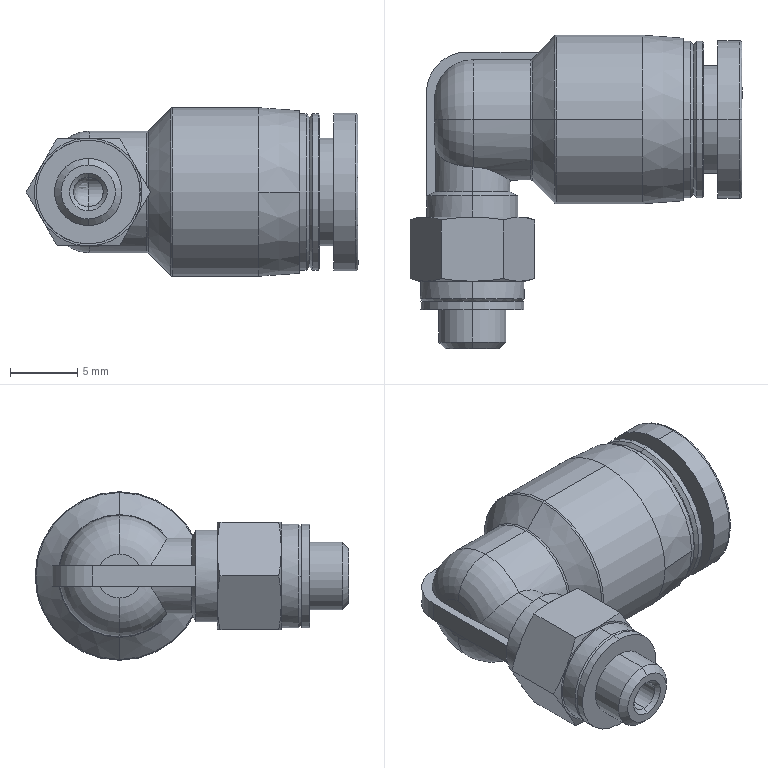Part | SolidWorks | features BaseBody 1 | 1 solid | 104 faces | box 24.619 x 23.25 x 12.5 mm | volume 2103 mm3 | cylinder 31 | cone 31 | plane 24 | spline 14 | torus 4 | commonest cylinder face diameters 2.2 x4 7.7 x4 11.6 x4 5.6 x3 6 x3 9 x3